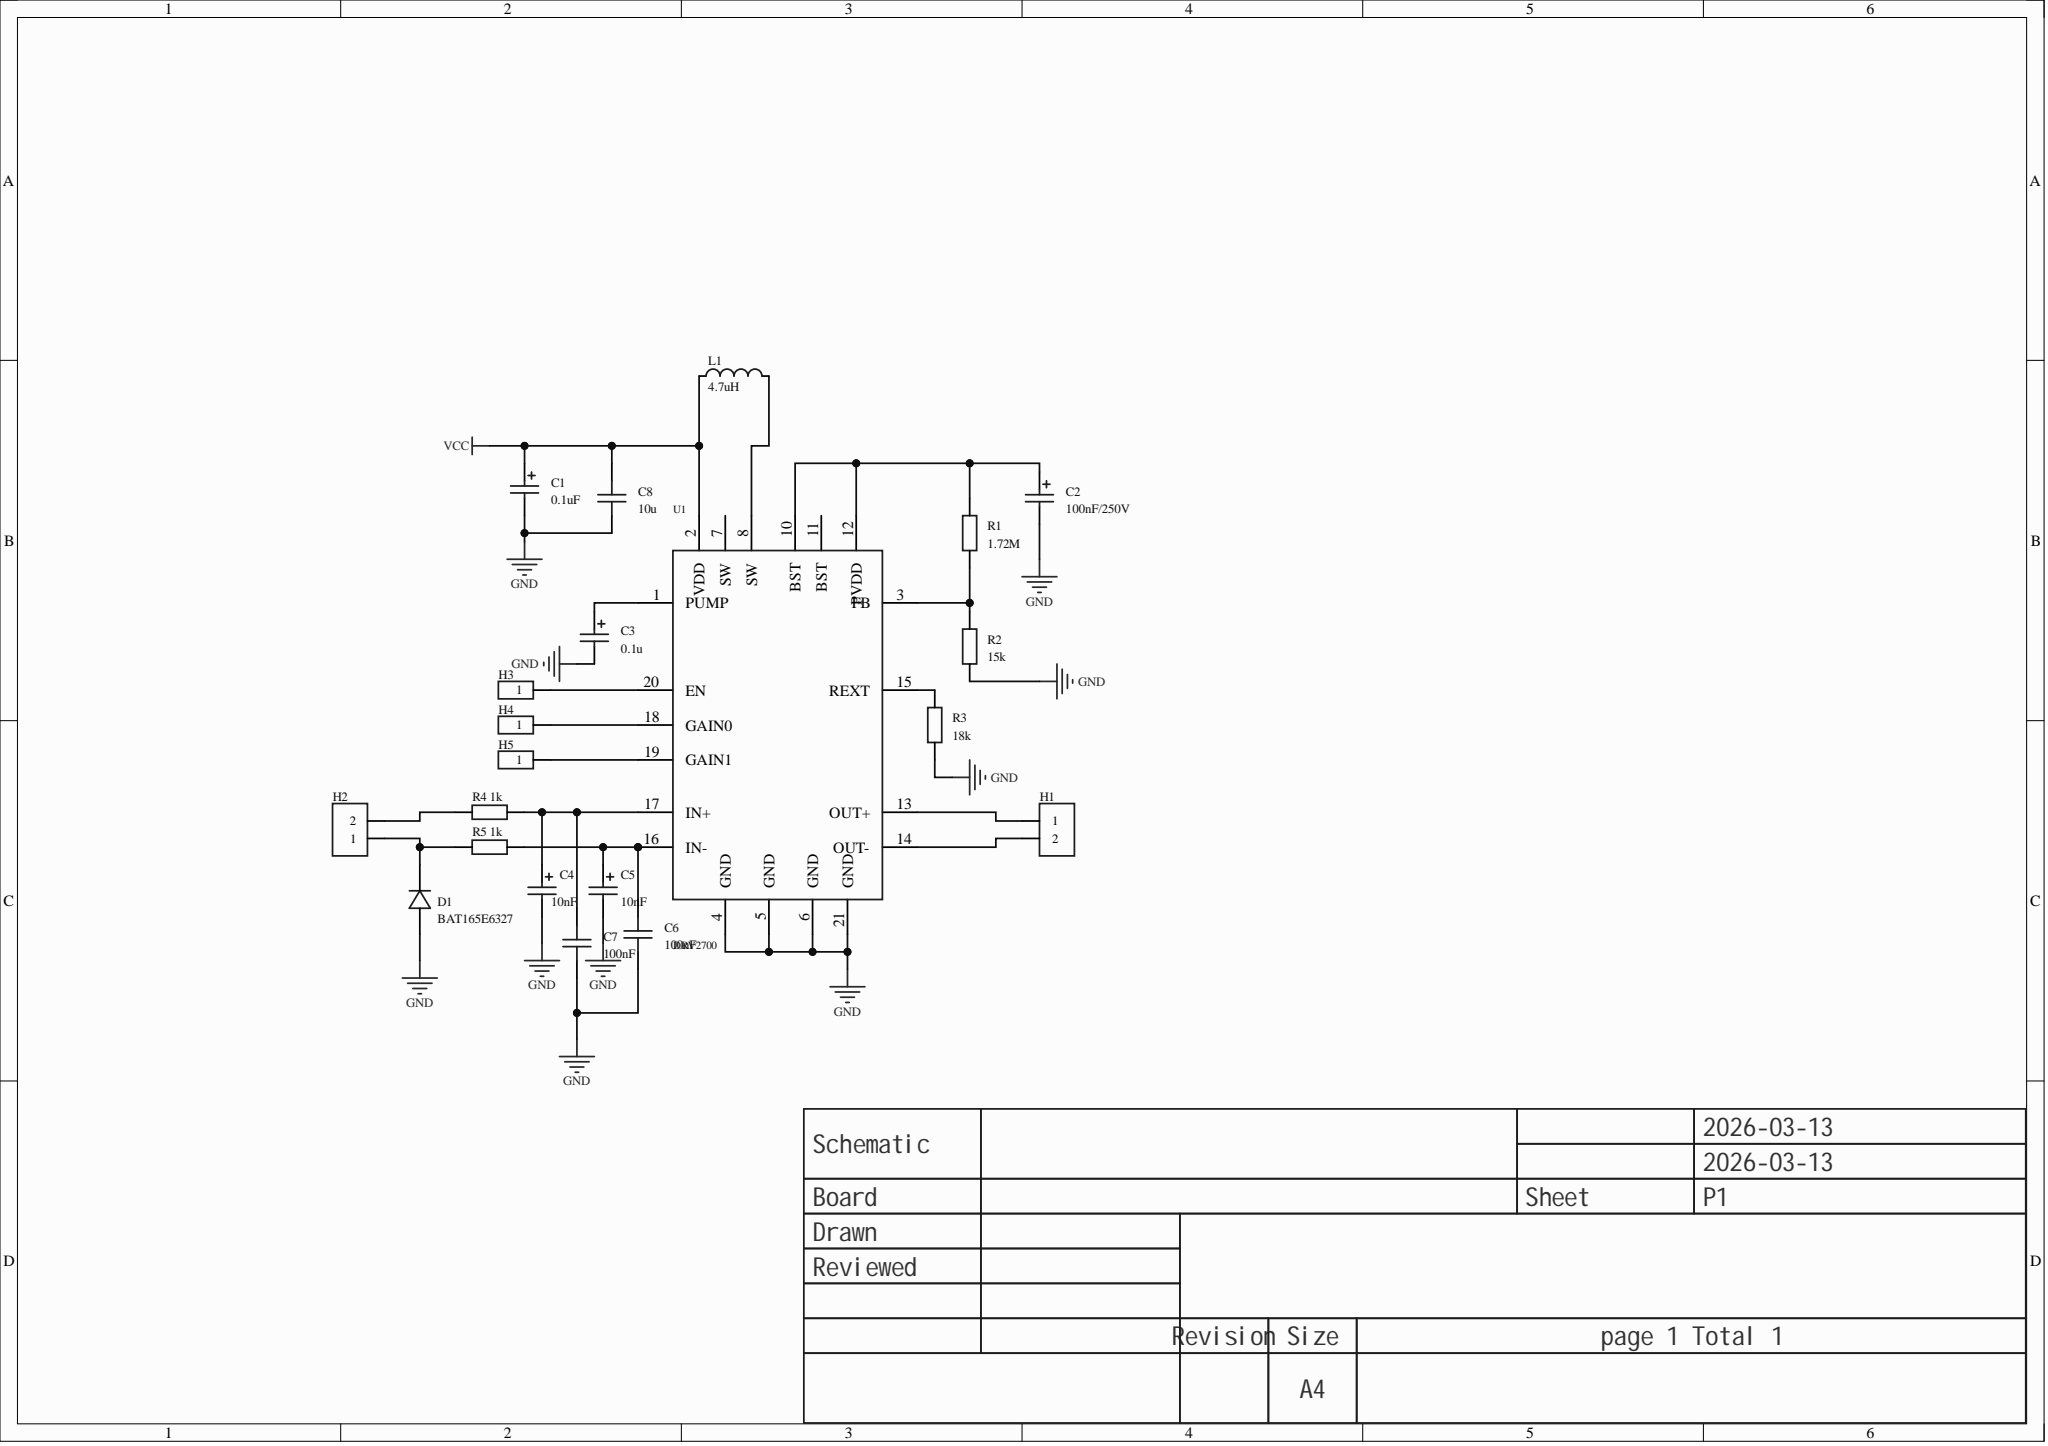Circuit board | Altium Designer | 21 parts | 16 nets
Bill of materials:
Comment,Description,Designator,Footprint,LibRef,Quantity
"0.1uF","","C1","C_Ele_SMD_3x5.4mm","C_Ele_SMD_3x5.4mm","1"
"100nF/250V","","C2","C_Ele_SMD_3x5.4mm","C_Ele_SMD_3x5.4mm","1"
"0.1u","","C3","C_Ele_SMD_3x5.4mm","C_Ele_SMD_3x5.4mm","1"
"10nF","","C4, C5","C_Ele_SMD_3x5.4mm","C_Ele_SMD_3x5.4mm","2"
"100nF","","C6, C7","C0805","CAP_0805","2"
"10u","","C8","C0805","CAP_0805","1"
"BAT165E6327","component BAT165E6327 compon Diode configuration: 1 single; Forward voltage (Vf): 740mV@750mA; DC reverse voltage (Vr): 40V; Rectifier current: 750mA;","D1","SOD-323_L1.8-W1.3-LS2.5-RD","BAT165E6327","1"
"","","H1, H2","HDR-TH_2P-P2.54-V-F","HDR-F_2.54_1x2P","2"
"","","H3, H4, H5","HDR-TH_1P-V-M_XKB_X4611WV-01I-C28D40","HDR-M_2.54_1x1P","3"
"4.7uH","component SRG0420-4R7-M comp Inductance: 4.7uH; Tolerance: ±20%; Rated current: 3A; Saturation current (Isat): 3.5A; Type: molded inductor;","L1","IND-SMD_L4.6-W4.1-A","SRG0420-4R7-M","1"
"1.72M","","R1","Res_1W","Res_AXIAL-1W","1"
"15k","","R2","Res_1W","Res_AXIAL-1W","1"
"18k","","R3","Res_1/4W","Res_AXIAL-1W","1"
"1k","","R4, R5","Res_1/4W","Res_AXIAL-1W","2"
"DRV2700","","U1","TI-RGP20-2700X2700TP_V","DRV2700","1"
Netlist (Protel format):
[
C1
C_Ele_SMD_3x5.4mm
0.1uF



]
[
C2
C_Ele_SMD_3x5.4mm
100nF/250V



]
[
C3
C_Ele_SMD_3x5.4mm
0.1u



]
[
C4
C_Ele_SMD_3x5.4mm
10nF



]
[
C5
C_Ele_SMD_3x5.4mm
10nF



]
[
C6
C0805
100nF



]
[
C7
C0805
100nF



]
[
C8
C0805
10u



]
[
D1
SOD-323_L1.8-W1.3-LS2.5-RD
BAT165E6327



]
[
H1
HDR-TH_2P-P2.54-V-F




]
[
H2
HDR-TH_2P-P2.54-V-F




]
[
H3
HDR-TH_1P-V-M_XKB_X4611WV-01I-C28D40




]
[
H4
HDR-TH_1P-V-M_XKB_X4611WV-01I-C28D40




]
[
H5
HDR-TH_1P-V-M_XKB_X4611WV-01I-C28D40




]
[
L1
IND-SMD_L4.6-W4.1-A
4.7uH



]
[
R1
Res_1W
1.72M



]
[
R2
Res_1W
15k



]
[
R3
Res_1/4W
18k



]
[
R4
Res_1/4W
1k



]
[
R5
Res_1/4W
1k



]
[
U1
TI-RGP20-2700X2700TP_V
DRV2700



]
(
VCC
C1-1
C8-2
L1-1
U1-2
)
(
NetR3_2
R3-2
U1-15
)
(
NetR1_1
R1-1
R2-2
U1-3
)
(
NetL1_2
L1-2
U1-8
)
(
NetH5_1
H5-1
U1-19
)
(
NetH4_1
H4-1
U1-18
)
(
NetH3_1
H3-1
U1-20
)
(
NetH2_2
H2-2
R4-1
)
(
NetH1_2
H1-2
U1-14
)
(
NetH1_1
H1-1
U1-13
)
(
NetD1_1
D1-1
H2-1
R5-1
)
(
NetC5_1
C5-1
C6-2
R5-2
U1-16
)
(
NetC4_1
C4-1
C7-2
R4-2
U1-17
)
(
NetC3_1
C3-1
U1-1
)
(
NetC2_1
C2-1
R1-2
U1-10
U1-12
)
(
GND
C1-2
C2-2
C3-2
C4-2
C5-2
C6-1
C7-1
C8-1
D1-2
R2-1
R3-1
U1-4
U1-5
U1-6
U1-21
)